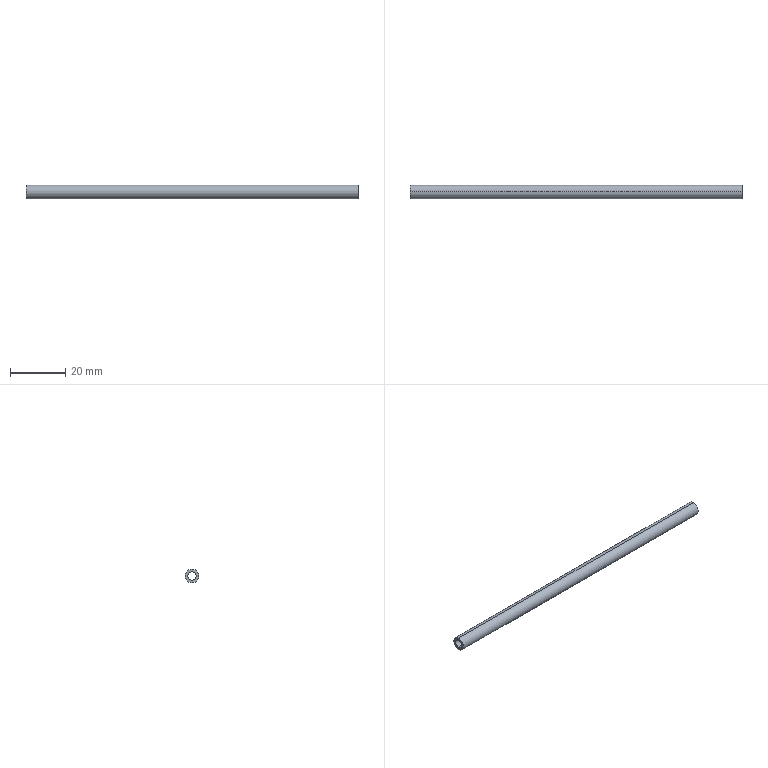Part | SolidWorks | features Extrusion 1 | 1 solid | 6 faces | box 120 x 5 x 5 mm | volume 1508 mm3 | cylinder 4 | plane 2 | commonest cylinder face diameters 3 x2 5 x2
STEP:
#1=CARTESIAN_POINT('',(120.,0.,1.5));
#2=VERTEX_POINT('',#1);
#3=CARTESIAN_POINT('',(120.,0.,-1.5));
#4=VERTEX_POINT('',#3);
#5=CARTESIAN_POINT('',(120.,0.,0.));
#6=DIRECTION('',(1.,0.,0.));
#7=DIRECTION('',(0.,0.,-1.));
#8=AXIS2_PLACEMENT_3D('',#5,#6,#7);
#9=CIRCLE('',#8,1.5);
#10=EDGE_CURVE('',#2,#4,#9,.T.);
#11=ORIENTED_EDGE('',*,*,#10,.T.);
#12=CARTESIAN_POINT('',(0.,0.,-1.5));
#13=VERTEX_POINT('',#12);
#14=CARTESIAN_POINT('',(120.,0.,-1.5));
#15=DIRECTION('',(-1.,0.,0.));
#16=VECTOR('',#15,1000.);
#17=LINE('',#14,#16);
#18=EDGE_CURVE('',#4,#13,#17,.T.);
#19=ORIENTED_EDGE('',*,*,#18,.T.);
#20=CARTESIAN_POINT('',(0.,0.,1.5));
#21=VERTEX_POINT('',#20);
#22=CARTESIAN_POINT('',(0.,0.,0.));
#23=DIRECTION('',(1.,0.,0.));
#24=DIRECTION('',(0.,0.,-1.));
#25=AXIS2_PLACEMENT_3D('',#22,#23,#24);
#26=CIRCLE('',#25,1.5);
#27=EDGE_CURVE('',#21,#13,#26,.T.);
#28=ORIENTED_EDGE('',*,*,#27,.F.);
#29=CARTESIAN_POINT('',(120.,0.,1.5));
#30=DIRECTION('',(-1.,0.,0.));
#31=VECTOR('',#30,1000.);
#32=LINE('',#29,#31);
#33=EDGE_CURVE('',#2,#21,#32,.T.);
#34=ORIENTED_EDGE('',*,*,#33,.F.);
#35=EDGE_LOOP('',(#11,#19,#28,#34));
#36=FACE_OUTER_BOUND('',#35,.T.);
#37=CARTESIAN_POINT('',(120.,0.,0.));
#38=DIRECTION('',(-1.,0.,0.));
#39=DIRECTION('',(0.,0.,1.));
#40=AXIS2_PLACEMENT_3D('',#37,#38,#39);
#41=CYLINDRICAL_SURFACE('',#40,1.5);
#42=ADVANCED_FACE('',(#36),#41,.F.);
#43=CARTESIAN_POINT('',(120.,0.,-2.5));
#44=VERTEX_POINT('',#43);
#45=CARTESIAN_POINT('',(120.,0.,2.5));
#46=VERTEX_POINT('',#45);
#47=CARTESIAN_POINT('',(120.,0.,0.));
#48=DIRECTION('',(1.,0.,0.));
#49=DIRECTION('',(0.,0.,-1.));
#50=AXIS2_PLACEMENT_3D('',#47,#48,#49);
#51=CIRCLE('',#50,2.5);
#52=EDGE_CURVE('',#44,#46,#51,.T.);
#53=ORIENTED_EDGE('',*,*,#52,.F.);
#54=CARTESIAN_POINT('',(0.,0.,-2.5));
#55=VERTEX_POINT('',#54);
#56=CARTESIAN_POINT('',(120.,0.,-2.5));
#57=DIRECTION('',(-1.,0.,0.));
#58=VECTOR('',#57,1000.);
#59=LINE('',#56,#58);
#60=EDGE_CURVE('',#44,#55,#59,.T.);
#61=ORIENTED_EDGE('',*,*,#60,.T.);
#62=CARTESIAN_POINT('',(0.,0.,2.5));
#63=VERTEX_POINT('',#62);
#64=CARTESIAN_POINT('',(0.,0.,0.));
#65=DIRECTION('',(1.,0.,0.));
#66=DIRECTION('',(0.,0.,-1.));
#67=AXIS2_PLACEMENT_3D('',#64,#65,#66);
#68=CIRCLE('',#67,2.5);
#69=EDGE_CURVE('',#55,#63,#68,.T.);
#70=ORIENTED_EDGE('',*,*,#69,.T.);
#71=CARTESIAN_POINT('',(120.,0.,2.5));
#72=DIRECTION('',(-1.,0.,0.));
#73=VECTOR('',#72,1000.);
#74=LINE('',#71,#73);
#75=EDGE_CURVE('',#46,#63,#74,.T.);
#76=ORIENTED_EDGE('',*,*,#75,.F.);
#77=EDGE_LOOP('',(#53,#61,#70,#76));
#78=FACE_OUTER_BOUND('',#77,.T.);
#79=CARTESIAN_POINT('',(120.,0.,0.));
#80=DIRECTION('',(-1.,0.,0.));
#81=DIRECTION('',(0.,0.,1.));
#82=AXIS2_PLACEMENT_3D('',#79,#80,#81);
#83=CYLINDRICAL_SURFACE('',#82,2.5);
#84=ADVANCED_FACE('',(#78),#83,.T.);
#85=CARTESIAN_POINT('',(120.,0.,0.));
#86=DIRECTION('',(1.,0.,0.));
#87=DIRECTION('',(0.,0.,-1.));
#88=AXIS2_PLACEMENT_3D('',#85,#86,#87);
#89=CIRCLE('',#88,2.5);
#90=EDGE_CURVE('',#46,#44,#89,.T.);
#91=ORIENTED_EDGE('',*,*,#90,.T.);
#92=ORIENTED_EDGE('',*,*,#52,.T.);
#93=EDGE_LOOP('',(#91,#92));
#94=FACE_OUTER_BOUND('',#93,.T.);
#95=ORIENTED_EDGE('',*,*,#10,.F.);
#96=CARTESIAN_POINT('',(120.,0.,0.));
#97=DIRECTION('',(1.,0.,0.));
#98=DIRECTION('',(0.,0.,-1.));
#99=AXIS2_PLACEMENT_3D('',#96,#97,#98);
#100=CIRCLE('',#99,1.5);
#101=EDGE_CURVE('',#4,#2,#100,.T.);
#102=ORIENTED_EDGE('',*,*,#101,.F.);
#103=EDGE_LOOP('',(#95,#102));
#104=FACE_BOUND('',#103,.T.);
#105=CARTESIAN_POINT('',(120.,0.,0.));
#106=DIRECTION('',(1.,0.,0.));
#107=DIRECTION('',(0.,0.,-1.));
#108=AXIS2_PLACEMENT_3D('',#105,#106,#107);
#109=PLANE('',#108);
#110=ADVANCED_FACE('',(#94,#104),#109,.T.);
#111=CARTESIAN_POINT('',(0.,0.,0.));
#112=DIRECTION('',(1.,0.,0.));
#113=DIRECTION('',(0.,0.,-1.));
#114=AXIS2_PLACEMENT_3D('',#111,#112,#113);
#115=CIRCLE('',#114,2.5);
#116=EDGE_CURVE('',#63,#55,#115,.T.);
#117=ORIENTED_EDGE('',*,*,#116,.F.);
#118=ORIENTED_EDGE('',*,*,#69,.F.);
#119=EDGE_LOOP('',(#117,#118));
#120=FACE_OUTER_BOUND('',#119,.T.);
#121=ORIENTED_EDGE('',*,*,#27,.T.);
#122=CARTESIAN_POINT('',(0.,0.,0.));
#123=DIRECTION('',(1.,0.,0.));
#124=DIRECTION('',(0.,0.,-1.));
#125=AXIS2_PLACEMENT_3D('',#122,#123,#124);
#126=CIRCLE('',#125,1.5);
#127=EDGE_CURVE('',#13,#21,#126,.T.);
#128=ORIENTED_EDGE('',*,*,#127,.T.);
#129=EDGE_LOOP('',(#121,#128));
#130=FACE_BOUND('',#129,.T.);
#131=CARTESIAN_POINT('',(0.,0.,0.));
#132=DIRECTION('',(1.,0.,0.));
#133=DIRECTION('',(0.,0.,-1.));
#134=AXIS2_PLACEMENT_3D('',#131,#132,#133);
#135=PLANE('',#134);
#136=ADVANCED_FACE('',(#120,#130),#135,.F.);
#137=ORIENTED_EDGE('',*,*,#60,.F.);
#138=ORIENTED_EDGE('',*,*,#90,.F.);
#139=ORIENTED_EDGE('',*,*,#75,.T.);
#140=ORIENTED_EDGE('',*,*,#116,.T.);
#141=EDGE_LOOP('',(#137,#138,#139,#140));
#142=FACE_OUTER_BOUND('',#141,.T.);
#143=CARTESIAN_POINT('',(120.,0.,0.));
#144=DIRECTION('',(-1.,0.,0.));
#145=DIRECTION('',(0.,0.,1.));
#146=AXIS2_PLACEMENT_3D('',#143,#144,#145);
#147=CYLINDRICAL_SURFACE('',#146,2.5);
#148=ADVANCED_FACE('',(#142),#147,.T.);
#149=ORIENTED_EDGE('',*,*,#18,.F.);
#150=ORIENTED_EDGE('',*,*,#101,.T.);
#151=ORIENTED_EDGE('',*,*,#33,.T.);
#152=ORIENTED_EDGE('',*,*,#127,.F.);
#153=EDGE_LOOP('',(#149,#150,#151,#152));
#154=FACE_OUTER_BOUND('',#153,.T.);
#155=CARTESIAN_POINT('',(120.,0.,0.));
#156=DIRECTION('',(-1.,0.,0.));
#157=DIRECTION('',(0.,0.,1.));
#158=AXIS2_PLACEMENT_3D('',#155,#156,#157);
#159=CYLINDRICAL_SURFACE('',#158,1.5);
#160=ADVANCED_FACE('',(#154),#159,.F.);
#161=CLOSED_SHELL('',(#42,#84,#110,#136,#148,#160));
#162=MANIFOLD_SOLID_BREP('',#161);
#163=CARTESIAN_POINT('',(0.,0.,0.));
#164=DIRECTION('',(0.,0.,1.));
#165=DIRECTION('',(1.,0.,0.));
#166=AXIS2_PLACEMENT_3D('',#163,#164,#165);
#167=(LENGTH_UNIT()NAMED_UNIT(*)SI_UNIT(.MILLI.,.METRE.));
#168=UNCERTAINTY_MEASURE_WITH_UNIT(LENGTH_MEASURE(0.00001),#167,'','');
#169=(NAMED_UNIT(*)PLANE_ANGLE_UNIT()SI_UNIT($,.RADIAN.));
#170=(NAMED_UNIT(*)SI_UNIT($,.STERADIAN.)SOLID_ANGLE_UNIT());
#171=(GEOMETRIC_REPRESENTATION_CONTEXT(3)GLOBAL_UNCERTAINTY_ASSIGNED_CONTEXT((#168))GLOBAL_UNIT_ASSIGNED_CONTEXT((#167,#169,#170))REPRESENTATION_CONTEXT('',''));
#172=ADVANCED_BREP_SHAPE_REPRESENTATION('',(#162,#166),#171);